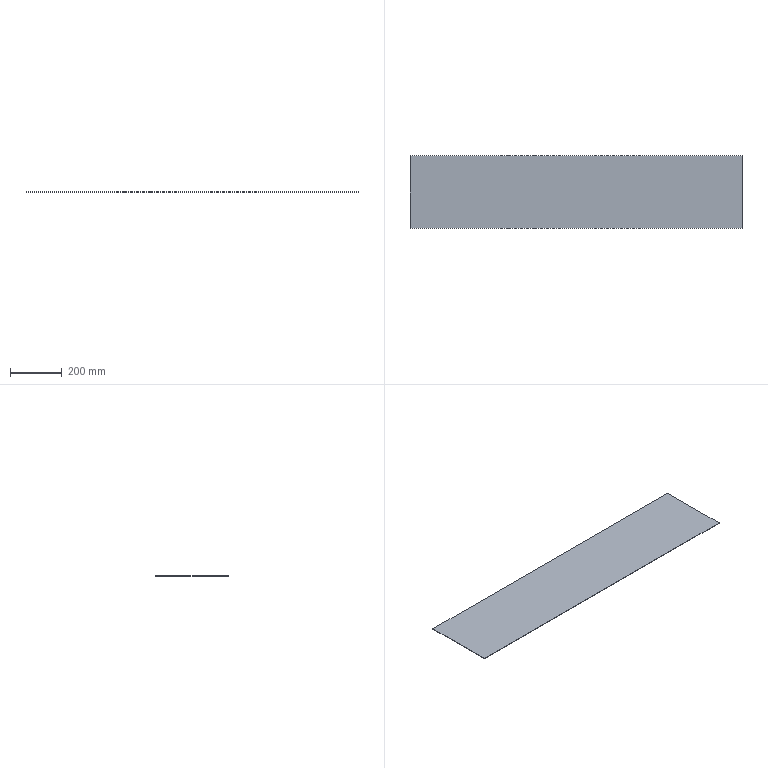Part | SolidWorks | features BaseBody 1 | 1 solid | 6 faces | box 1280 x 280 x 1.5 mm | volume 537600 mm3 | plane 6
STEP:
#1=CARTESIAN_POINT('',(640.,0.,0.));
#2=VERTEX_POINT('',#1);
#3=CARTESIAN_POINT('',(640.,280.,0.));
#4=VERTEX_POINT('',#3);
#5=CARTESIAN_POINT('',(640.,280.,0.));
#6=DIRECTION('',(0.,1.,0.));
#7=VECTOR('',#6,1000.);
#8=LINE('',#5,#7);
#9=EDGE_CURVE('',#2,#4,#8,.T.);
#10=ORIENTED_EDGE('',*,*,#9,.T.);
#11=CARTESIAN_POINT('',(-640.,280.,0.));
#12=VERTEX_POINT('',#11);
#13=CARTESIAN_POINT('',(-640.,280.,0.));
#14=DIRECTION('',(-1.,0.,0.));
#15=VECTOR('',#14,1000.);
#16=LINE('',#13,#15);
#17=EDGE_CURVE('',#4,#12,#16,.T.);
#18=ORIENTED_EDGE('',*,*,#17,.T.);
#19=CARTESIAN_POINT('',(-640.,0.,0.));
#20=VERTEX_POINT('',#19);
#21=CARTESIAN_POINT('',(-640.,280.,0.));
#22=DIRECTION('',(0.,-1.,0.));
#23=VECTOR('',#22,1000.);
#24=LINE('',#21,#23);
#25=EDGE_CURVE('',#12,#20,#24,.T.);
#26=ORIENTED_EDGE('',*,*,#25,.T.);
#27=CARTESIAN_POINT('',(640.,0.,0.));
#28=DIRECTION('',(1.,0.,0.));
#29=VECTOR('',#28,1000.);
#30=LINE('',#27,#29);
#31=EDGE_CURVE('',#20,#2,#30,.T.);
#32=ORIENTED_EDGE('',*,*,#31,.T.);
#33=EDGE_LOOP('',(#10,#18,#26,#32));
#34=FACE_OUTER_BOUND('',#33,.T.);
#35=CARTESIAN_POINT('',(0.,0.,0.));
#36=DIRECTION('',(0.,0.,-1.));
#37=DIRECTION('',(0.,-1.,0.));
#38=AXIS2_PLACEMENT_3D('',#35,#36,#37);
#39=PLANE('',#38);
#40=ADVANCED_FACE('',(#34),#39,.F.);
#41=CARTESIAN_POINT('',(640.,0.,-1.5));
#42=VERTEX_POINT('',#41);
#43=CARTESIAN_POINT('',(640.,280.,-1.5));
#44=VERTEX_POINT('',#43);
#45=CARTESIAN_POINT('',(640.,280.,-1.5));
#46=DIRECTION('',(0.,1.,0.));
#47=VECTOR('',#46,1000.);
#48=LINE('',#45,#47);
#49=EDGE_CURVE('',#42,#44,#48,.T.);
#50=ORIENTED_EDGE('',*,*,#49,.F.);
#51=CARTESIAN_POINT('',(-640.,0.,-1.5));
#52=VERTEX_POINT('',#51);
#53=CARTESIAN_POINT('',(640.,0.,-1.5));
#54=DIRECTION('',(1.,0.,0.));
#55=VECTOR('',#54,1000.);
#56=LINE('',#53,#55);
#57=EDGE_CURVE('',#52,#42,#56,.T.);
#58=ORIENTED_EDGE('',*,*,#57,.F.);
#59=CARTESIAN_POINT('',(-640.,280.,-1.5));
#60=VERTEX_POINT('',#59);
#61=CARTESIAN_POINT('',(-640.,280.,-1.5));
#62=DIRECTION('',(0.,-1.,0.));
#63=VECTOR('',#62,1000.);
#64=LINE('',#61,#63);
#65=EDGE_CURVE('',#60,#52,#64,.T.);
#66=ORIENTED_EDGE('',*,*,#65,.F.);
#67=CARTESIAN_POINT('',(-640.,280.,-1.5));
#68=DIRECTION('',(-1.,0.,0.));
#69=VECTOR('',#68,1000.);
#70=LINE('',#67,#69);
#71=EDGE_CURVE('',#44,#60,#70,.T.);
#72=ORIENTED_EDGE('',*,*,#71,.F.);
#73=EDGE_LOOP('',(#50,#58,#66,#72));
#74=FACE_OUTER_BOUND('',#73,.T.);
#75=CARTESIAN_POINT('',(0.,0.,-1.5));
#76=DIRECTION('',(0.,0.,-1.));
#77=DIRECTION('',(0.,-1.,0.));
#78=AXIS2_PLACEMENT_3D('',#75,#76,#77);
#79=PLANE('',#78);
#80=ADVANCED_FACE('',(#74),#79,.T.);
#81=ORIENTED_EDGE('',*,*,#17,.F.);
#82=CARTESIAN_POINT('',(640.,280.,-1.5));
#83=DIRECTION('',(0.,0.,1.));
#84=VECTOR('',#83,1000.);
#85=LINE('',#82,#84);
#86=EDGE_CURVE('',#44,#4,#85,.T.);
#87=ORIENTED_EDGE('',*,*,#86,.F.);
#88=ORIENTED_EDGE('',*,*,#71,.T.);
#89=CARTESIAN_POINT('',(-640.,280.,-1.5));
#90=DIRECTION('',(0.,0.,1.));
#91=VECTOR('',#90,1000.);
#92=LINE('',#89,#91);
#93=EDGE_CURVE('',#60,#12,#92,.T.);
#94=ORIENTED_EDGE('',*,*,#93,.T.);
#95=EDGE_LOOP('',(#81,#87,#88,#94));
#96=FACE_OUTER_BOUND('',#95,.T.);
#97=CARTESIAN_POINT('',(-640.,280.,-1.5));
#98=DIRECTION('',(0.,1.,0.));
#99=DIRECTION('',(1.,0.,0.));
#100=AXIS2_PLACEMENT_3D('',#97,#98,#99);
#101=PLANE('',#100);
#102=ADVANCED_FACE('',(#96),#101,.T.);
#103=ORIENTED_EDGE('',*,*,#25,.F.);
#104=ORIENTED_EDGE('',*,*,#93,.F.);
#105=ORIENTED_EDGE('',*,*,#65,.T.);
#106=CARTESIAN_POINT('',(-640.,0.,-1.5));
#107=DIRECTION('',(0.,0.,1.));
#108=VECTOR('',#107,1000.);
#109=LINE('',#106,#108);
#110=EDGE_CURVE('',#52,#20,#109,.T.);
#111=ORIENTED_EDGE('',*,*,#110,.T.);
#112=EDGE_LOOP('',(#103,#104,#105,#111));
#113=FACE_OUTER_BOUND('',#112,.T.);
#114=CARTESIAN_POINT('',(-640.,280.,-1.5));
#115=DIRECTION('',(-1.,0.,0.));
#116=DIRECTION('',(0.,0.,1.));
#117=AXIS2_PLACEMENT_3D('',#114,#115,#116);
#118=PLANE('',#117);
#119=ADVANCED_FACE('',(#113),#118,.T.);
#120=ORIENTED_EDGE('',*,*,#31,.F.);
#121=ORIENTED_EDGE('',*,*,#110,.F.);
#122=ORIENTED_EDGE('',*,*,#57,.T.);
#123=CARTESIAN_POINT('',(640.,0.,-1.5));
#124=DIRECTION('',(0.,0.,1.));
#125=VECTOR('',#124,1000.);
#126=LINE('',#123,#125);
#127=EDGE_CURVE('',#42,#2,#126,.T.);
#128=ORIENTED_EDGE('',*,*,#127,.T.);
#129=EDGE_LOOP('',(#120,#121,#122,#128));
#130=FACE_OUTER_BOUND('',#129,.T.);
#131=CARTESIAN_POINT('',(640.,0.,-1.5));
#132=DIRECTION('',(0.,-1.,0.));
#133=DIRECTION('',(0.,0.,-1.));
#134=AXIS2_PLACEMENT_3D('',#131,#132,#133);
#135=PLANE('',#134);
#136=ADVANCED_FACE('',(#130),#135,.T.);
#137=ORIENTED_EDGE('',*,*,#9,.F.);
#138=ORIENTED_EDGE('',*,*,#127,.F.);
#139=ORIENTED_EDGE('',*,*,#49,.T.);
#140=ORIENTED_EDGE('',*,*,#86,.T.);
#141=EDGE_LOOP('',(#137,#138,#139,#140));
#142=FACE_OUTER_BOUND('',#141,.T.);
#143=CARTESIAN_POINT('',(640.,280.,-1.5));
#144=DIRECTION('',(1.,0.,0.));
#145=DIRECTION('',(0.,1.,0.));
#146=AXIS2_PLACEMENT_3D('',#143,#144,#145);
#147=PLANE('',#146);
#148=ADVANCED_FACE('',(#142),#147,.T.);
#149=CLOSED_SHELL('',(#40,#80,#102,#119,#136,#148));
#150=MANIFOLD_SOLID_BREP('',#149);
#151=CARTESIAN_POINT('',(0.,0.,0.));
#152=DIRECTION('',(0.,0.,1.));
#153=DIRECTION('',(1.,0.,0.));
#154=AXIS2_PLACEMENT_3D('',#151,#152,#153);
#155=(LENGTH_UNIT()NAMED_UNIT(*)SI_UNIT(.MILLI.,.METRE.));
#156=UNCERTAINTY_MEASURE_WITH_UNIT(LENGTH_MEASURE(0.00001),#155,'','');
#157=(NAMED_UNIT(*)PLANE_ANGLE_UNIT()SI_UNIT($,.RADIAN.));
#158=(NAMED_UNIT(*)SI_UNIT($,.STERADIAN.)SOLID_ANGLE_UNIT());
#159=(GEOMETRIC_REPRESENTATION_CONTEXT(3)GLOBAL_UNCERTAINTY_ASSIGNED_CONTEXT((#156))GLOBAL_UNIT_ASSIGNED_CONTEXT((#155,#157,#158))REPRESENTATION_CONTEXT('',''));
#160=ADVANCED_BREP_SHAPE_REPRESENTATION('',(#150,#154),#159);